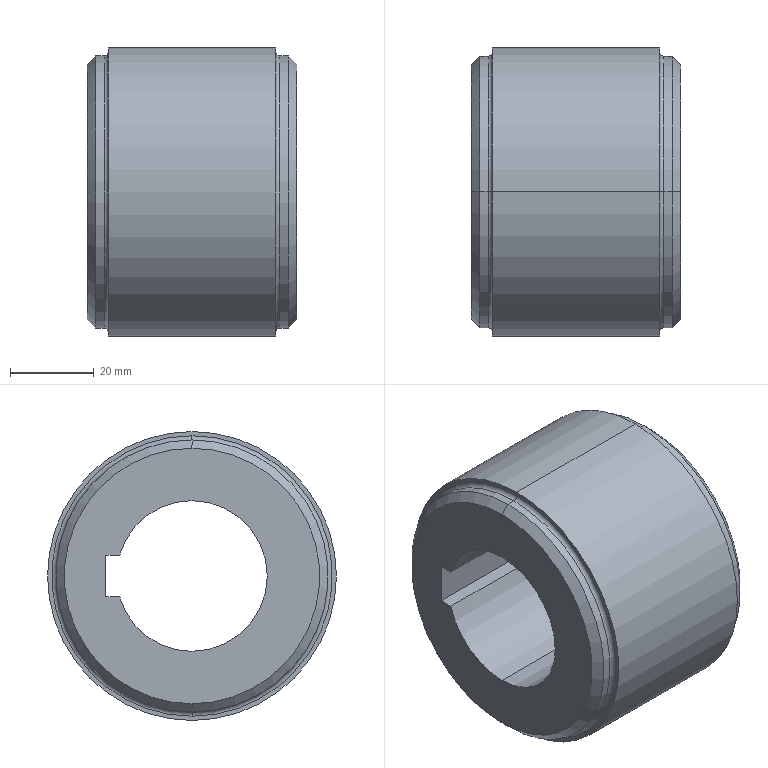Part | SolidWorks | features Chamfer 1, Extrusion 1, Fillet 1, ICE 1 | 1 solid | 24 faces | box 50 x 69 x 69 mm | volume 129736 mm3 | cylinder 9 | plane 7 | cone 4 | torus 4 | commonest cylinder face diameters 65 x4 36 x3 69 x2
STEP:
#1=CARTESIAN_POINT('',(-25.,0.,30.5));
#2=VERTEX_POINT('',#1);
#3=CARTESIAN_POINT('',(-25.,0.,-30.5));
#4=VERTEX_POINT('',#3);
#5=CARTESIAN_POINT('',(-25.,0.,0.));
#6=DIRECTION('',(-1.,0.,0.));
#7=DIRECTION('',(0.,0.,-1.));
#8=AXIS2_PLACEMENT_3D('',#5,#6,#7);
#9=CIRCLE('',#8,30.5);
#10=EDGE_CURVE('',#2,#4,#9,.T.);
#11=ORIENTED_EDGE('',*,*,#10,.F.);
#12=CARTESIAN_POINT('',(-23.,0.,32.5));
#13=VERTEX_POINT('',#12);
#14=CARTESIAN_POINT('',(-23.,0.,32.5));
#15=DIRECTION('',(0.7071,0.,0.7071));
#16=VECTOR('',#15,1000.);
#17=LINE('',#14,#16);
#18=EDGE_CURVE('',#2,#13,#17,.T.);
#19=ORIENTED_EDGE('',*,*,#18,.T.);
#20=CARTESIAN_POINT('',(-23.,0.,-32.5));
#21=VERTEX_POINT('',#20);
#22=CARTESIAN_POINT('',(-23.,0.,0.));
#23=DIRECTION('',(1.,0.,0.));
#24=DIRECTION('',(0.,0.,-1.));
#25=AXIS2_PLACEMENT_3D('',#22,#23,#24);
#26=CIRCLE('',#25,32.5);
#27=EDGE_CURVE('',#21,#13,#26,.T.);
#28=ORIENTED_EDGE('',*,*,#27,.F.);
#29=CARTESIAN_POINT('',(-23.,0.,-32.5));
#30=DIRECTION('',(0.7071,0.,-0.7071));
#31=VECTOR('',#30,1000.);
#32=LINE('',#29,#31);
#33=EDGE_CURVE('',#4,#21,#32,.T.);
#34=ORIENTED_EDGE('',*,*,#33,.F.);
#35=EDGE_LOOP('',(#11,#19,#28,#34));
#36=FACE_OUTER_BOUND('',#35,.T.);
#37=CARTESIAN_POINT('',(-23.,0.,0.));
#38=DIRECTION('',(1.,0.,0.));
#39=DIRECTION('',(0.,0.,-1.));
#40=AXIS2_PLACEMENT_3D('',#37,#38,#39);
#41=CONICAL_SURFACE('',#40,32.5,0.7854);
#42=ADVANCED_FACE('',(#36),#41,.T.);
#43=CARTESIAN_POINT('',(25.,0.,-30.5));
#44=VERTEX_POINT('',#43);
#45=CARTESIAN_POINT('',(25.,0.,30.5));
#46=VERTEX_POINT('',#45);
#47=CARTESIAN_POINT('',(25.,0.,0.));
#48=DIRECTION('',(1.,0.,0.));
#49=DIRECTION('',(0.,0.,-1.));
#50=AXIS2_PLACEMENT_3D('',#47,#48,#49);
#51=CIRCLE('',#50,30.5);
#52=EDGE_CURVE('',#44,#46,#51,.T.);
#53=ORIENTED_EDGE('',*,*,#52,.F.);
#54=CARTESIAN_POINT('',(23.,0.,-32.5));
#55=VERTEX_POINT('',#54);
#56=CARTESIAN_POINT('',(25.,0.,-30.5));
#57=DIRECTION('',(-0.7071,0.,-0.7071));
#58=VECTOR('',#57,1000.);
#59=LINE('',#56,#58);
#60=EDGE_CURVE('',#44,#55,#59,.T.);
#61=ORIENTED_EDGE('',*,*,#60,.T.);
#62=CARTESIAN_POINT('',(23.,0.,32.5));
#63=VERTEX_POINT('',#62);
#64=CARTESIAN_POINT('',(23.,0.,0.));
#65=DIRECTION('',(-1.,0.,0.));
#66=DIRECTION('',(0.,0.,-1.));
#67=AXIS2_PLACEMENT_3D('',#64,#65,#66);
#68=CIRCLE('',#67,32.5);
#69=EDGE_CURVE('',#63,#55,#68,.T.);
#70=ORIENTED_EDGE('',*,*,#69,.F.);
#71=CARTESIAN_POINT('',(25.,0.,30.5));
#72=DIRECTION('',(-0.7071,0.,0.7071));
#73=VECTOR('',#72,1000.);
#74=LINE('',#71,#73);
#75=EDGE_CURVE('',#46,#63,#74,.T.);
#76=ORIENTED_EDGE('',*,*,#75,.F.);
#77=EDGE_LOOP('',(#53,#61,#70,#76));
#78=FACE_OUTER_BOUND('',#77,.T.);
#79=CARTESIAN_POINT('',(25.,0.,0.));
#80=DIRECTION('',(-1.,0.,0.));
#81=DIRECTION('',(0.,0.,1.));
#82=AXIS2_PLACEMENT_3D('',#79,#80,#81);
#83=CONICAL_SURFACE('',#82,30.5,0.7854);
#84=ADVANCED_FACE('',(#78),#83,.T.);
#85=CARTESIAN_POINT('',(21.,0.,32.5));
#86=VERTEX_POINT('',#85);
#87=CARTESIAN_POINT('',(21.,0.,-32.5));
#88=VERTEX_POINT('',#87);
#89=CARTESIAN_POINT('',(21.,0.,0.));
#90=DIRECTION('',(1.,0.,0.));
#91=DIRECTION('',(0.,0.,-1.));
#92=AXIS2_PLACEMENT_3D('',#89,#90,#91);
#93=CIRCLE('',#92,32.5);
#94=EDGE_CURVE('',#86,#88,#93,.T.);
#95=ORIENTED_EDGE('',*,*,#94,.F.);
#96=CARTESIAN_POINT('',(20.,0.,33.5));
#97=VERTEX_POINT('',#96);
#98=CARTESIAN_POINT('',(21.,0.,33.5));
#99=DIRECTION('',(0.,1.,0.));
#100=DIRECTION('',(0.,0.,1.));
#101=AXIS2_PLACEMENT_3D('',#98,#99,#100);
#102=CIRCLE('',#101,1.);
#103=EDGE_CURVE('',#86,#97,#102,.T.);
#104=ORIENTED_EDGE('',*,*,#103,.T.);
#105=CARTESIAN_POINT('',(20.,0.,-33.5));
#106=VERTEX_POINT('',#105);
#107=CARTESIAN_POINT('',(20.,0.,0.));
#108=DIRECTION('',(-1.,0.,0.));
#109=DIRECTION('',(0.,0.,-1.));
#110=AXIS2_PLACEMENT_3D('',#107,#108,#109);
#111=CIRCLE('',#110,33.5);
#112=EDGE_CURVE('',#106,#97,#111,.T.);
#113=ORIENTED_EDGE('',*,*,#112,.F.);
#114=CARTESIAN_POINT('',(21.,0.,-33.5));
#115=DIRECTION('',(0.,-1.,0.));
#116=DIRECTION('',(0.,0.,-1.));
#117=AXIS2_PLACEMENT_3D('',#114,#115,#116);
#118=CIRCLE('',#117,1.);
#119=EDGE_CURVE('',#88,#106,#118,.T.);
#120=ORIENTED_EDGE('',*,*,#119,.F.);
#121=EDGE_LOOP('',(#95,#104,#113,#120));
#122=FACE_OUTER_BOUND('',#121,.T.);
#123=CARTESIAN_POINT('',(21.,0.,0.));
#124=DIRECTION('',(1.,0.,0.));
#125=DIRECTION('',(0.,0.,-1.));
#126=AXIS2_PLACEMENT_3D('',#123,#124,#125);
#127=TOROIDAL_SURFACE('',#126,33.5,1.);
#128=ADVANCED_FACE('',(#122),#127,.F.);
#129=CARTESIAN_POINT('',(-20.,0.,33.5));
#130=VERTEX_POINT('',#129);
#131=CARTESIAN_POINT('',(-20.,0.,-33.5));
#132=VERTEX_POINT('',#131);
#133=CARTESIAN_POINT('',(-20.,0.,0.));
#134=DIRECTION('',(1.,0.,0.));
#135=DIRECTION('',(0.,0.,-1.));
#136=AXIS2_PLACEMENT_3D('',#133,#134,#135);
#137=CIRCLE('',#136,33.5);
#138=EDGE_CURVE('',#130,#132,#137,.T.);
#139=ORIENTED_EDGE('',*,*,#138,.F.);
#140=CARTESIAN_POINT('',(-21.,0.,32.5));
#141=VERTEX_POINT('',#140);
#142=CARTESIAN_POINT('',(-21.,0.,33.5));
#143=DIRECTION('',(0.,1.,0.));
#144=DIRECTION('',(0.,0.,1.));
#145=AXIS2_PLACEMENT_3D('',#142,#143,#144);
#146=CIRCLE('',#145,1.);
#147=EDGE_CURVE('',#130,#141,#146,.T.);
#148=ORIENTED_EDGE('',*,*,#147,.T.);
#149=CARTESIAN_POINT('',(-21.,0.,-32.5));
#150=VERTEX_POINT('',#149);
#151=CARTESIAN_POINT('',(-21.,0.,0.));
#152=DIRECTION('',(-1.,0.,0.));
#153=DIRECTION('',(0.,0.,-1.));
#154=AXIS2_PLACEMENT_3D('',#151,#152,#153);
#155=CIRCLE('',#154,32.5);
#156=EDGE_CURVE('',#150,#141,#155,.T.);
#157=ORIENTED_EDGE('',*,*,#156,.F.);
#158=CARTESIAN_POINT('',(-21.,0.,-33.5));
#159=DIRECTION('',(0.,-1.,0.));
#160=DIRECTION('',(0.,0.,-1.));
#161=AXIS2_PLACEMENT_3D('',#158,#159,#160);
#162=CIRCLE('',#161,1.);
#163=EDGE_CURVE('',#132,#150,#162,.T.);
#164=ORIENTED_EDGE('',*,*,#163,.F.);
#165=EDGE_LOOP('',(#139,#148,#157,#164));
#166=FACE_OUTER_BOUND('',#165,.T.);
#167=CARTESIAN_POINT('',(-21.,0.,0.));
#168=DIRECTION('',(1.,0.,0.));
#169=DIRECTION('',(0.,0.,-1.));
#170=AXIS2_PLACEMENT_3D('',#167,#168,#169);
#171=TOROIDAL_SURFACE('',#170,33.5,1.);
#172=ADVANCED_FACE('',(#166),#171,.F.);
#173=CARTESIAN_POINT('',(20.,0.,-34.5));
#174=VERTEX_POINT('',#173);
#175=CARTESIAN_POINT('',(20.,0.,34.5));
#176=VERTEX_POINT('',#175);
#177=CARTESIAN_POINT('',(20.,0.,0.));
#178=DIRECTION('',(1.,0.,0.));
#179=DIRECTION('',(0.,0.,-1.));
#180=AXIS2_PLACEMENT_3D('',#177,#178,#179);
#181=CIRCLE('',#180,34.5);
#182=EDGE_CURVE('',#174,#176,#181,.T.);
#183=ORIENTED_EDGE('',*,*,#182,.F.);
#184=CARTESIAN_POINT('',(-20.,0.,-34.5));
#185=VERTEX_POINT('',#184);
#186=CARTESIAN_POINT('',(20.,0.,-34.5));
#187=DIRECTION('',(-1.,0.,0.));
#188=VECTOR('',#187,1000.);
#189=LINE('',#186,#188);
#190=EDGE_CURVE('',#174,#185,#189,.T.);
#191=ORIENTED_EDGE('',*,*,#190,.T.);
#192=CARTESIAN_POINT('',(-20.,0.,34.5));
#193=VERTEX_POINT('',#192);
#194=CARTESIAN_POINT('',(-20.,0.,0.));
#195=DIRECTION('',(1.,0.,0.));
#196=DIRECTION('',(0.,0.,-1.));
#197=AXIS2_PLACEMENT_3D('',#194,#195,#196);
#198=CIRCLE('',#197,34.5);
#199=EDGE_CURVE('',#185,#193,#198,.T.);
#200=ORIENTED_EDGE('',*,*,#199,.T.);
#201=CARTESIAN_POINT('',(20.,0.,34.5));
#202=DIRECTION('',(-1.,0.,0.));
#203=VECTOR('',#202,1000.);
#204=LINE('',#201,#203);
#205=EDGE_CURVE('',#176,#193,#204,.T.);
#206=ORIENTED_EDGE('',*,*,#205,.F.);
#207=EDGE_LOOP('',(#183,#191,#200,#206));
#208=FACE_OUTER_BOUND('',#207,.T.);
#209=CARTESIAN_POINT('',(20.,0.,0.));
#210=DIRECTION('',(-1.,0.,0.));
#211=DIRECTION('',(0.,0.,1.));
#212=AXIS2_PLACEMENT_3D('',#209,#210,#211);
#213=CYLINDRICAL_SURFACE('',#212,34.5);
#214=ADVANCED_FACE('',(#208),#213,.T.);
#215=CARTESIAN_POINT('',(25.,0.,18.));
#216=VERTEX_POINT('',#215);
#217=CARTESIAN_POINT('',(25.,0.,-18.));
#218=VERTEX_POINT('',#217);
#219=CARTESIAN_POINT('',(25.,0.,0.));
#220=DIRECTION('',(1.,0.,0.));
#221=DIRECTION('',(0.,0.,-1.));
#222=AXIS2_PLACEMENT_3D('',#219,#220,#221);
#223=CIRCLE('',#222,18.);
#224=EDGE_CURVE('',#216,#218,#223,.T.);
#225=ORIENTED_EDGE('',*,*,#224,.T.);
#226=CARTESIAN_POINT('',(-25.,0.,-18.));
#227=VERTEX_POINT('',#226);
#228=CARTESIAN_POINT('',(25.,0.,-18.));
#229=DIRECTION('',(-1.,0.,0.));
#230=VECTOR('',#229,1000.);
#231=LINE('',#228,#230);
#232=EDGE_CURVE('',#218,#227,#231,.T.);
#233=ORIENTED_EDGE('',*,*,#232,.T.);
#234=CARTESIAN_POINT('',(-25.,0.,18.));
#235=VERTEX_POINT('',#234);
#236=CARTESIAN_POINT('',(-25.,0.,0.));
#237=DIRECTION('',(1.,0.,0.));
#238=DIRECTION('',(0.,0.,-1.));
#239=AXIS2_PLACEMENT_3D('',#236,#237,#238);
#240=CIRCLE('',#239,18.);
#241=EDGE_CURVE('',#235,#227,#240,.T.);
#242=ORIENTED_EDGE('',*,*,#241,.F.);
#243=CARTESIAN_POINT('',(25.,0.,18.));
#244=DIRECTION('',(-1.,0.,0.));
#245=VECTOR('',#244,1000.);
#246=LINE('',#243,#245);
#247=EDGE_CURVE('',#216,#235,#246,.T.);
#248=ORIENTED_EDGE('',*,*,#247,.F.);
#249=EDGE_LOOP('',(#225,#233,#242,#248));
#250=FACE_OUTER_BOUND('',#249,.T.);
#251=CARTESIAN_POINT('',(25.,0.,0.));
#252=DIRECTION('',(-1.,0.,0.));
#253=DIRECTION('',(0.,0.,1.));
#254=AXIS2_PLACEMENT_3D('',#251,#252,#253);
#255=CYLINDRICAL_SURFACE('',#254,18.);
#256=ADVANCED_FACE('',(#250),#255,.F.);
#257=CARTESIAN_POINT('',(25.,17.292,5.));
#258=VERTEX_POINT('',#257);
#259=CARTESIAN_POINT('',(25.,0.,0.));
#260=DIRECTION('',(1.,0.,0.));
#261=DIRECTION('',(0.,0.,-1.));
#262=AXIS2_PLACEMENT_3D('',#259,#260,#261);
#263=CIRCLE('',#262,18.);
#264=EDGE_CURVE('',#258,#216,#263,.T.);
#265=ORIENTED_EDGE('',*,*,#264,.T.);
#266=ORIENTED_EDGE('',*,*,#247,.T.);
#267=CARTESIAN_POINT('',(-25.,17.292,5.));
#268=VERTEX_POINT('',#267);
#269=CARTESIAN_POINT('',(-25.,0.,0.));
#270=DIRECTION('',(1.,0.,0.));
#271=DIRECTION('',(0.,0.,-1.));
#272=AXIS2_PLACEMENT_3D('',#269,#270,#271);
#273=CIRCLE('',#272,18.);
#274=EDGE_CURVE('',#268,#235,#273,.T.);
#275=ORIENTED_EDGE('',*,*,#274,.F.);
#276=CARTESIAN_POINT('',(25.,17.292,5.));
#277=DIRECTION('',(-1.,0.,0.));
#278=VECTOR('',#277,1000.);
#279=LINE('',#276,#278);
#280=EDGE_CURVE('',#258,#268,#279,.T.);
#281=ORIENTED_EDGE('',*,*,#280,.F.);
#282=EDGE_LOOP('',(#265,#266,#275,#281));
#283=FACE_OUTER_BOUND('',#282,.T.);
#284=CARTESIAN_POINT('',(25.,0.,0.));
#285=DIRECTION('',(-1.,0.,0.));
#286=DIRECTION('',(0.,0.,1.));
#287=AXIS2_PLACEMENT_3D('',#284,#285,#286);
#288=CYLINDRICAL_SURFACE('',#287,18.);
#289=ADVANCED_FACE('',(#283),#288,.F.);
#290=ORIENTED_EDGE('',*,*,#69,.T.);
#291=CARTESIAN_POINT('',(25.,0.,-32.5));
#292=DIRECTION('',(-1.,0.,0.));
#293=VECTOR('',#292,1000.);
#294=LINE('',#291,#293);
#295=EDGE_CURVE('',#55,#88,#294,.T.);
#296=ORIENTED_EDGE('',*,*,#295,.T.);
#297=CARTESIAN_POINT('',(21.,0.,0.));
#298=DIRECTION('',(1.,0.,0.));
#299=DIRECTION('',(0.,0.,-1.));
#300=AXIS2_PLACEMENT_3D('',#297,#298,#299);
#301=CIRCLE('',#300,32.5);
#302=EDGE_CURVE('',#88,#86,#301,.T.);
#303=ORIENTED_EDGE('',*,*,#302,.T.);
#304=CARTESIAN_POINT('',(25.,0.,32.5));
#305=DIRECTION('',(-1.,0.,0.));
#306=VECTOR('',#305,1000.);
#307=LINE('',#304,#306);
#308=EDGE_CURVE('',#63,#86,#307,.T.);
#309=ORIENTED_EDGE('',*,*,#308,.F.);
#310=EDGE_LOOP('',(#290,#296,#303,#309));
#311=FACE_OUTER_BOUND('',#310,.T.);
#312=CARTESIAN_POINT('',(25.,0.,0.));
#313=DIRECTION('',(-1.,0.,0.));
#314=DIRECTION('',(0.,0.,1.));
#315=AXIS2_PLACEMENT_3D('',#312,#313,#314);
#316=CYLINDRICAL_SURFACE('',#315,32.5);
#317=ADVANCED_FACE('',(#311),#316,.T.);
#318=CARTESIAN_POINT('',(-21.,0.,0.));
#319=DIRECTION('',(-1.,0.,0.));
#320=DIRECTION('',(0.,0.,-1.));
#321=AXIS2_PLACEMENT_3D('',#318,#319,#320);
#322=CIRCLE('',#321,32.5);
#323=EDGE_CURVE('',#141,#150,#322,.T.);
#324=ORIENTED_EDGE('',*,*,#323,.T.);
#325=CARTESIAN_POINT('',(25.,0.,-32.5));
#326=DIRECTION('',(-1.,0.,0.));
#327=VECTOR('',#326,1000.);
#328=LINE('',#325,#327);
#329=EDGE_CURVE('',#150,#21,#328,.T.);
#330=ORIENTED_EDGE('',*,*,#329,.T.);
#331=ORIENTED_EDGE('',*,*,#27,.T.);
#332=CARTESIAN_POINT('',(25.,0.,32.5));
#333=DIRECTION('',(-1.,0.,0.));
#334=VECTOR('',#333,1000.);
#335=LINE('',#332,#334);
#336=EDGE_CURVE('',#141,#13,#335,.T.);
#337=ORIENTED_EDGE('',*,*,#336,.F.);
#338=EDGE_LOOP('',(#324,#330,#331,#337));
#339=FACE_OUTER_BOUND('',#338,.T.);
#340=CARTESIAN_POINT('',(25.,0.,0.));
#341=DIRECTION('',(-1.,0.,0.));
#342=DIRECTION('',(0.,0.,1.));
#343=AXIS2_PLACEMENT_3D('',#340,#341,#342);
#344=CYLINDRICAL_SURFACE('',#343,32.5);
#345=ADVANCED_FACE('',(#339),#344,.T.);
#346=ORIENTED_EDGE('',*,*,#329,.F.);
#347=ORIENTED_EDGE('',*,*,#156,.T.);
#348=ORIENTED_EDGE('',*,*,#336,.T.);
#349=CARTESIAN_POINT('',(-23.,0.,0.));
#350=DIRECTION('',(1.,0.,0.));
#351=DIRECTION('',(0.,0.,-1.));
#352=AXIS2_PLACEMENT_3D('',#349,#350,#351);
#353=CIRCLE('',#352,32.5);
#354=EDGE_CURVE('',#13,#21,#353,.T.);
#355=ORIENTED_EDGE('',*,*,#354,.T.);
#356=EDGE_LOOP('',(#346,#347,#348,#355));
#357=FACE_OUTER_BOUND('',#356,.T.);
#358=CARTESIAN_POINT('',(25.,0.,0.));
#359=DIRECTION('',(-1.,0.,0.));
#360=DIRECTION('',(0.,0.,1.));
#361=AXIS2_PLACEMENT_3D('',#358,#359,#360);
#362=CYLINDRICAL_SURFACE('',#361,32.5);
#363=ADVANCED_FACE('',(#357),#362,.T.);
#364=CARTESIAN_POINT('',(25.,0.,0.));
#365=DIRECTION('',(1.,0.,0.));
#366=DIRECTION('',(0.,0.,-1.));
#367=AXIS2_PLACEMENT_3D('',#364,#365,#366);
#368=CIRCLE('',#367,30.5);
#369=EDGE_CURVE('',#46,#44,#368,.T.);
#370=ORIENTED_EDGE('',*,*,#369,.T.);
#371=ORIENTED_EDGE('',*,*,#52,.T.);
#372=EDGE_LOOP('',(#370,#371));
#373=FACE_OUTER_BOUND('',#372,.T.);
#374=CARTESIAN_POINT('',(25.,17.292,-5.));
#375=VERTEX_POINT('',#374);
#376=CARTESIAN_POINT('',(25.,20.592,-5.));
#377=VERTEX_POINT('',#376);
#378=CARTESIAN_POINT('',(25.,17.292,-5.));
#379=DIRECTION('',(0.,1.,0.));
#380=VECTOR('',#379,1000.);
#381=LINE('',#378,#380);
#382=EDGE_CURVE('',#375,#377,#381,.T.);
#383=ORIENTED_EDGE('',*,*,#382,.F.);
#384=CARTESIAN_POINT('',(25.,0.,0.));
#385=DIRECTION('',(1.,0.,0.));
#386=DIRECTION('',(0.,0.,-1.));
#387=AXIS2_PLACEMENT_3D('',#384,#385,#386);
#388=CIRCLE('',#387,18.);
#389=EDGE_CURVE('',#218,#375,#388,.T.);
#390=ORIENTED_EDGE('',*,*,#389,.F.);
#391=ORIENTED_EDGE('',*,*,#224,.F.);
#392=ORIENTED_EDGE('',*,*,#264,.F.);
#393=CARTESIAN_POINT('',(25.,20.592,5.));
#394=VERTEX_POINT('',#393);
#395=CARTESIAN_POINT('',(25.,20.592,5.));
#396=DIRECTION('',(0.,-1.,0.));
#397=VECTOR('',#396,1000.);
#398=LINE('',#395,#397);
#399=EDGE_CURVE('',#394,#258,#398,.T.);
#400=ORIENTED_EDGE('',*,*,#399,.F.);
#401=CARTESIAN_POINT('',(25.,20.592,-5.));
#402=DIRECTION('',(0.,0.,1.));
#403=VECTOR('',#402,1000.);
#404=LINE('',#401,#403);
#405=EDGE_CURVE('',#377,#394,#404,.T.);
#406=ORIENTED_EDGE('',*,*,#405,.F.);
#407=EDGE_LOOP('',(#383,#390,#391,#392,#400,#406));
#408=FACE_BOUND('',#407,.T.);
#409=CARTESIAN_POINT('',(25.,0.,0.));
#410=DIRECTION('',(1.,0.,0.));
#411=DIRECTION('',(0.,0.,-1.));
#412=AXIS2_PLACEMENT_3D('',#409,#410,#411);
#413=PLANE('',#412);
#414=ADVANCED_FACE('',(#373,#408),#413,.T.);
#415=CARTESIAN_POINT('',(-25.,0.,0.));
#416=DIRECTION('',(-1.,0.,0.));
#417=DIRECTION('',(0.,0.,-1.));
#418=AXIS2_PLACEMENT_3D('',#415,#416,#417);
#419=CIRCLE('',#418,30.5);
#420=EDGE_CURVE('',#4,#2,#419,.T.);
#421=ORIENTED_EDGE('',*,*,#420,.T.);
#422=ORIENTED_EDGE('',*,*,#10,.T.);
#423=EDGE_LOOP('',(#421,#422));
#424=FACE_OUTER_BOUND('',#423,.T.);
#425=ORIENTED_EDGE('',*,*,#274,.T.);
#426=ORIENTED_EDGE('',*,*,#241,.T.);
#427=CARTESIAN_POINT('',(-25.,17.292,-5.));
#428=VERTEX_POINT('',#427);
#429=CARTESIAN_POINT('',(-25.,0.,0.));
#430=DIRECTION('',(1.,0.,0.));
#431=DIRECTION('',(0.,0.,-1.));
#432=AXIS2_PLACEMENT_3D('',#429,#430,#431);
#433=CIRCLE('',#432,18.);
#434=EDGE_CURVE('',#227,#428,#433,.T.);
#435=ORIENTED_EDGE('',*,*,#434,.T.);
#436=CARTESIAN_POINT('',(-25.,20.592,-5.));
#437=VERTEX_POINT('',#436);
#438=CARTESIAN_POINT('',(-25.,17.292,-5.));
#439=DIRECTION('',(0.,1.,0.));
#440=VECTOR('',#439,1000.);
#441=LINE('',#438,#440);
#442=EDGE_CURVE('',#428,#437,#441,.T.);
#443=ORIENTED_EDGE('',*,*,#442,.T.);
#444=CARTESIAN_POINT('',(-25.,20.592,5.));
#445=VERTEX_POINT('',#444);
#446=CARTESIAN_POINT('',(-25.,20.592,-5.));
#447=DIRECTION('',(0.,0.,1.));
#448=VECTOR('',#447,1000.);
#449=LINE('',#446,#448);
#450=EDGE_CURVE('',#437,#445,#449,.T.);
#451=ORIENTED_EDGE('',*,*,#450,.T.);
#452=CARTESIAN_POINT('',(-25.,20.592,5.));
#453=DIRECTION('',(0.,-1.,0.));
#454=VECTOR('',#453,1000.);
#455=LINE('',#452,#454);
#456=EDGE_CURVE('',#445,#268,#455,.T.);
#457=ORIENTED_EDGE('',*,*,#456,.T.);
#458=EDGE_LOOP('',(#425,#426,#435,#443,#451,#457));
#459=FACE_BOUND('',#458,.T.);
#460=CARTESIAN_POINT('',(-25.,0.,0.));
#461=DIRECTION('',(1.,0.,0.));
#462=DIRECTION('',(0.,0.,-1.));
#463=AXIS2_PLACEMENT_3D('',#460,#461,#462);
#464=PLANE('',#463);
#465=ADVANCED_FACE('',(#424,#459),#464,.F.);
#466=ORIENTED_EDGE('',*,*,#295,.F.);
#467=CARTESIAN_POINT('',(23.,0.,0.));
#468=DIRECTION('',(-1.,0.,0.));
#469=DIRECTION('',(0.,0.,-1.));
#470=AXIS2_PLACEMENT_3D('',#467,#468,#469);
#471=CIRCLE('',#470,32.5);
#472=EDGE_CURVE('',#55,#63,#471,.T.);
#473=ORIENTED_EDGE('',*,*,#472,.T.);
#474=ORIENTED_EDGE('',*,*,#308,.T.);
#475=ORIENTED_EDGE('',*,*,#94,.T.);
#476=EDGE_LOOP('',(#466,#473,#474,#475));
#477=FACE_OUTER_BOUND('',#476,.T.);
#478=CARTESIAN_POINT('',(25.,0.,0.));
#479=DIRECTION('',(-1.,0.,0.));
#480=DIRECTION('',(0.,0.,1.));
#481=AXIS2_PLACEMENT_3D('',#478,#479,#480);
#482=CYLINDRICAL_SURFACE('',#481,32.5);
#483=ADVANCED_FACE('',(#477),#482,.T.);
#484=ORIENTED_EDGE('',*,*,#232,.F.);
#485=ORIENTED_EDGE('',*,*,#389,.T.);
#486=CARTESIAN_POINT('',(25.,17.292,-5.));
#487=DIRECTION('',(-1.,0.,0.));
#488=VECTOR('',#487,1000.);
#489=LINE('',#486,#488);
#490=EDGE_CURVE('',#375,#428,#489,.T.);
#491=ORIENTED_EDGE('',*,*,#490,.T.);
#492=ORIENTED_EDGE('',*,*,#434,.F.);
#493=EDGE_LOOP('',(#484,#485,#491,#492));
#494=FACE_OUTER_BOUND('',#493,.T.);
#495=CARTESIAN_POINT('',(25.,0.,0.));
#496=DIRECTION('',(-1.,0.,0.));
#497=DIRECTION('',(0.,0.,1.));
#498=AXIS2_PLACEMENT_3D('',#495,#496,#497);
#499=CYLINDRICAL_SURFACE('',#498,18.);
#500=ADVANCED_FACE('',(#494),#499,.F.);
#501=ORIENTED_EDGE('',*,*,#442,.F.);
#502=ORIENTED_EDGE('',*,*,#490,.F.);
#503=ORIENTED_EDGE('',*,*,#382,.T.);
#504=CARTESIAN_POINT('',(25.,20.592,-5.));
#505=DIRECTION('',(-1.,0.,0.));
#506=VECTOR('',#505,1000.);
#507=LINE('',#504,#506);
#508=EDGE_CURVE('',#377,#437,#507,.T.);
#509=ORIENTED_EDGE('',*,*,#508,.T.);
#510=EDGE_LOOP('',(#501,#502,#503,#509));
#511=FACE_OUTER_BOUND('',#510,.T.);
#512=CARTESIAN_POINT('',(25.,17.292,-5.));
#513=DIRECTION('',(0.,0.,1.));
#514=DIRECTION('',(0.,-1.,0.));
#515=AXIS2_PLACEMENT_3D('',#512,#513,#514);
#516=PLANE('',#515);
#517=ADVANCED_FACE('',(#511),#516,.T.);
#518=ORIENTED_EDGE('',*,*,#450,.F.);
#519=ORIENTED_EDGE('',*,*,#508,.F.);
#520=ORIENTED_EDGE('',*,*,#405,.T.);
#521=CARTESIAN_POINT('',(25.,20.592,5.));
#522=DIRECTION('',(-1.,0.,0.));
#523=VECTOR('',#522,1000.);
#524=LINE('',#521,#523);
#525=EDGE_CURVE('',#394,#445,#524,.T.);
#526=ORIENTED_EDGE('',*,*,#525,.T.);
#527=EDGE_LOOP('',(#518,#519,#520,#526));
#528=FACE_OUTER_BOUND('',#527,.T.);
#529=CARTESIAN_POINT('',(25.,20.592,-5.));
#530=DIRECTION('',(0.,-1.,0.));
#531=DIRECTION('',(0.,0.,-1.));
#532=AXIS2_PLACEMENT_3D('',#529,#530,#531);
#533=PLANE('',#532);
#534=ADVANCED_FACE('',(#528),#533,.T.);
#535=ORIENTED_EDGE('',*,*,#456,.F.);
#536=ORIENTED_EDGE('',*,*,#525,.F.);
#537=ORIENTED_EDGE('',*,*,#399,.T.);
#538=ORIENTED_EDGE('',*,*,#280,.T.);
#539=EDGE_LOOP('',(#535,#536,#537,#538));
#540=FACE_OUTER_BOUND('',#539,.T.);
#541=CARTESIAN_POINT('',(25.,20.592,5.));
#542=DIRECTION('',(0.,0.,-1.));
#543=DIRECTION('',(-1.,0.,0.));
#544=AXIS2_PLACEMENT_3D('',#541,#542,#543);
#545=PLANE('',#544);
#546=ADVANCED_FACE('',(#540),#545,.T.);
#547=ORIENTED_EDGE('',*,*,#112,.T.);
#548=CARTESIAN_POINT('',(20.,0.,0.));
#549=DIRECTION('',(-1.,0.,0.));
#550=DIRECTION('',(0.,0.,-1.));
#551=AXIS2_PLACEMENT_3D('',#548,#549,#550);
#552=CIRCLE('',#551,33.5);
#553=EDGE_CURVE('',#97,#106,#552,.T.);
#554=ORIENTED_EDGE('',*,*,#553,.T.);
#555=EDGE_LOOP('',(#547,#554));
#556=FACE_BOUND('',#555,.T.);
#557=CARTESIAN_POINT('',(20.,0.,0.));
#558=DIRECTION('',(1.,0.,0.));
#559=DIRECTION('',(0.,0.,-1.));
#560=AXIS2_PLACEMENT_3D('',#557,#558,#559);
#561=CIRCLE('',#560,34.5);
#562=EDGE_CURVE('',#176,#174,#561,.T.);
#563=ORIENTED_EDGE('',*,*,#562,.T.);
#564=ORIENTED_EDGE('',*,*,#182,.T.);
#565=EDGE_LOOP('',(#563,#564));
#566=FACE_OUTER_BOUND('',#565,.T.);
#567=CARTESIAN_POINT('',(20.,0.,0.));
#568=DIRECTION('',(1.,0.,0.));
#569=DIRECTION('',(0.,0.,-1.));
#570=AXIS2_PLACEMENT_3D('',#567,#568,#569);
#571=PLANE('',#570);
#572=ADVANCED_FACE('',(#556,#566),#571,.T.);
#573=CARTESIAN_POINT('',(-20.,0.,0.));
#574=DIRECTION('',(1.,0.,0.));
#575=DIRECTION('',(0.,0.,-1.));
#576=AXIS2_PLACEMENT_3D('',#573,#574,#575);
#577=CIRCLE('',#576,33.5);
#578=EDGE_CURVE('',#132,#130,#577,.T.);
#579=ORIENTED_EDGE('',*,*,#578,.T.);
#580=ORIENTED_EDGE('',*,*,#138,.T.);
#581=EDGE_LOOP('',(#579,#580));
#582=FACE_BOUND('',#581,.T.);
#583=CARTESIAN_POINT('',(-20.,0.,0.));
#584=DIRECTION('',(1.,0.,0.));
#585=DIRECTION('',(0.,0.,-1.));
#586=AXIS2_PLACEMENT_3D('',#583,#584,#585);
#587=CIRCLE('',#586,34.5);
#588=EDGE_CURVE('',#193,#185,#587,.T.);
#589=ORIENTED_EDGE('',*,*,#588,.F.);
#590=ORIENTED_EDGE('',*,*,#199,.F.);
#591=EDGE_LOOP('',(#589,#590));
#592=FACE_OUTER_BOUND('',#591,.T.);
#593=CARTESIAN_POINT('',(-20.,0.,0.));
#594=DIRECTION('',(1.,0.,0.));
#595=DIRECTION('',(0.,0.,-1.));
#596=AXIS2_PLACEMENT_3D('',#593,#594,#595);
#597=PLANE('',#596);
#598=ADVANCED_FACE('',(#582,#592),#597,.F.);
#599=ORIENTED_EDGE('',*,*,#190,.F.);
#600=ORIENTED_EDGE('',*,*,#562,.F.);
#601=ORIENTED_EDGE('',*,*,#205,.T.);
#602=ORIENTED_EDGE('',*,*,#588,.T.);
#603=EDGE_LOOP('',(#599,#600,#601,#602));
#604=FACE_OUTER_BOUND('',#603,.T.);
#605=CARTESIAN_POINT('',(20.,0.,0.));
#606=DIRECTION('',(-1.,0.,0.));
#607=DIRECTION('',(0.,0.,1.));
#608=AXIS2_PLACEMENT_3D('',#605,#606,#607);
#609=CYLINDRICAL_SURFACE('',#608,34.5);
#610=ADVANCED_FACE('',(#604),#609,.T.);
#611=ORIENTED_EDGE('',*,*,#147,.F.);
#612=ORIENTED_EDGE('',*,*,#578,.F.);
#613=ORIENTED_EDGE('',*,*,#163,.T.);
#614=ORIENTED_EDGE('',*,*,#323,.F.);
#615=EDGE_LOOP('',(#611,#612,#613,#614));
#616=FACE_OUTER_BOUND('',#615,.T.);
#617=CARTESIAN_POINT('',(-21.,0.,0.));
#618=DIRECTION('',(1.,0.,0.));
#619=DIRECTION('',(0.,0.,-1.));
#620=AXIS2_PLACEMENT_3D('',#617,#618,#619);
#621=TOROIDAL_SURFACE('',#620,33.5,1.);
#622=ADVANCED_FACE('',(#616),#621,.F.);
#623=ORIENTED_EDGE('',*,*,#103,.F.);
#624=ORIENTED_EDGE('',*,*,#302,.F.);
#625=ORIENTED_EDGE('',*,*,#119,.T.);
#626=ORIENTED_EDGE('',*,*,#553,.F.);
#627=EDGE_LOOP('',(#623,#624,#625,#626));
#628=FACE_OUTER_BOUND('',#627,.T.);
#629=CARTESIAN_POINT('',(21.,0.,0.));
#630=DIRECTION('',(1.,0.,0.));
#631=DIRECTION('',(0.,0.,-1.));
#632=AXIS2_PLACEMENT_3D('',#629,#630,#631);
#633=TOROIDAL_SURFACE('',#632,33.5,1.);
#634=ADVANCED_FACE('',(#628),#633,.F.);
#635=ORIENTED_EDGE('',*,*,#60,.F.);
#636=ORIENTED_EDGE('',*,*,#369,.F.);
#637=ORIENTED_EDGE('',*,*,#75,.T.);
#638=ORIENTED_EDGE('',*,*,#472,.F.);
#639=EDGE_LOOP('',(#635,#636,#637,#638));
#640=FACE_OUTER_BOUND('',#639,.T.);
#641=CARTESIAN_POINT('',(25.,0.,0.));
#642=DIRECTION('',(-1.,0.,0.));
#643=DIRECTION('',(0.,0.,1.));
#644=AXIS2_PLACEMENT_3D('',#641,#642,#643);
#645=CONICAL_SURFACE('',#644,30.5,0.7854);
#646=ADVANCED_FACE('',(#640),#645,.T.);
#647=ORIENTED_EDGE('',*,*,#18,.F.);
#648=ORIENTED_EDGE('',*,*,#420,.F.);
#649=ORIENTED_EDGE('',*,*,#33,.T.);
#650=ORIENTED_EDGE('',*,*,#354,.F.);
#651=EDGE_LOOP('',(#647,#648,#649,#650));
#652=FACE_OUTER_BOUND('',#651,.T.);
#653=CARTESIAN_POINT('',(-23.,0.,0.));
#654=DIRECTION('',(1.,0.,0.));
#655=DIRECTION('',(0.,0.,-1.));
#656=AXIS2_PLACEMENT_3D('',#653,#654,#655);
#657=CONICAL_SURFACE('',#656,32.5,0.7854);
#658=ADVANCED_FACE('',(#652),#657,.T.);
#659=CLOSED_SHELL('',(#42,#84,#128,#172,#214,#256,#289,#317,#345,#363,#414,#465,#483,#500,#517,#534,#546,#572,#598,#610,#622,#634,#646,#658));
#660=MANIFOLD_SOLID_BREP('',#659);
#661=CARTESIAN_POINT('',(0.,0.,0.));
#662=DIRECTION('',(0.,0.,1.));
#663=DIRECTION('',(1.,0.,0.));
#664=AXIS2_PLACEMENT_3D('',#661,#662,#663);
#665=(LENGTH_UNIT()NAMED_UNIT(*)SI_UNIT(.MILLI.,.METRE.));
#666=UNCERTAINTY_MEASURE_WITH_UNIT(LENGTH_MEASURE(0.00001),#665,'','');
#667=(NAMED_UNIT(*)PLANE_ANGLE_UNIT()SI_UNIT($,.RADIAN.));
#668=(NAMED_UNIT(*)SI_UNIT($,.STERADIAN.)SOLID_ANGLE_UNIT());
#669=(GEOMETRIC_REPRESENTATION_CONTEXT(3)GLOBAL_UNCERTAINTY_ASSIGNED_CONTEXT((#666))GLOBAL_UNIT_ASSIGNED_CONTEXT((#665,#667,#668))REPRESENTATION_CONTEXT('',''));
#670=ADVANCED_BREP_SHAPE_REPRESENTATION('',(#660,#664),#669);